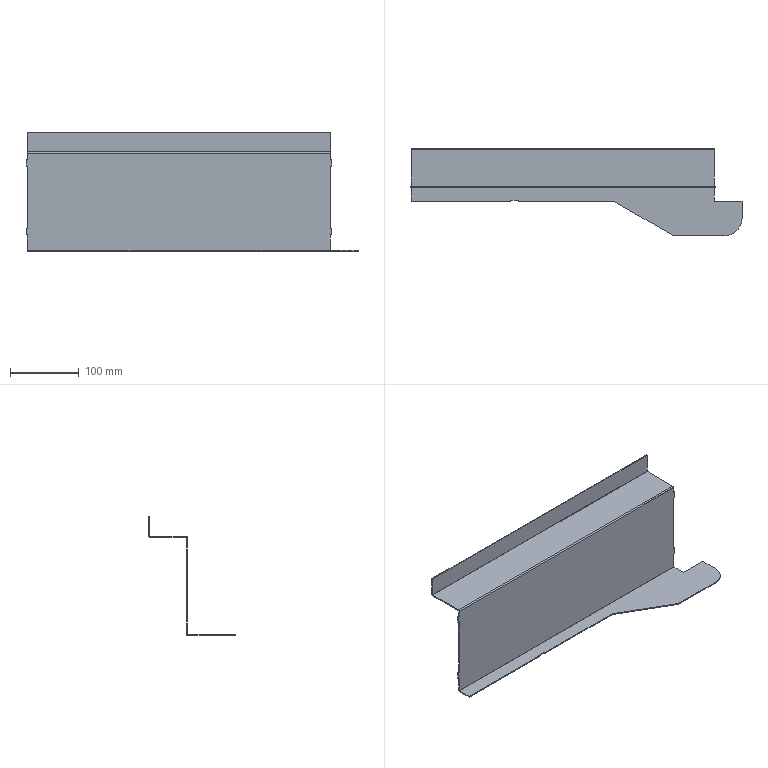Part | STEP file | FHD-021-001-K rack welded part K | 1 solid | 43 faces | box 482.9 x 126.5 x 173 mm | volume 173847 mm3 | plane 36 | cylinder 7 | commonest cylinder face diameters 0.4 x3 3.4 x3 50 x1